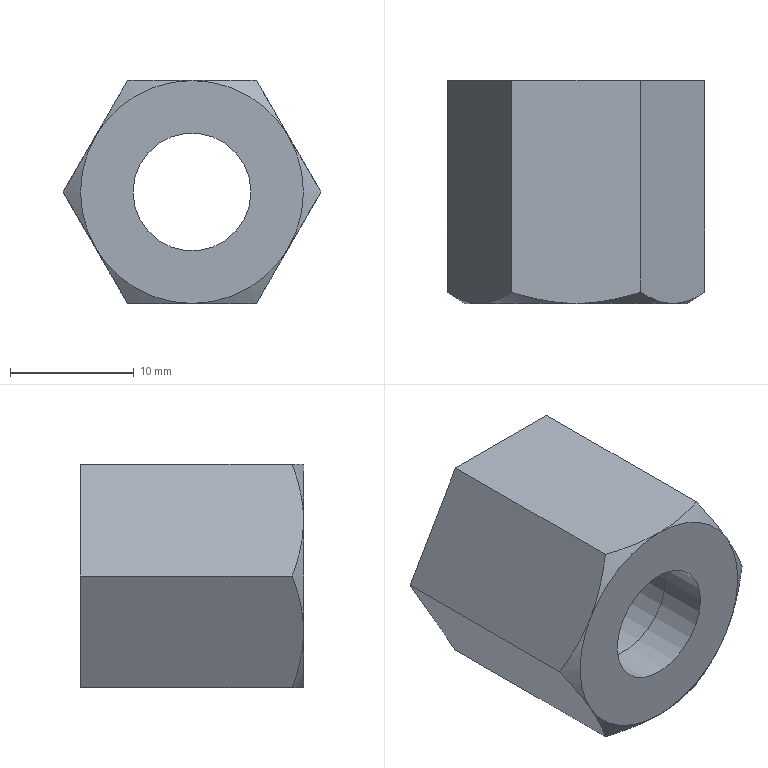Part | STEP file | 1-55.7 | 2 solids | 16 faces | box 20.785 x 18 x 18 mm | volume 3019 mm3 | plane 11 | cylinder 4 | cone 1 | commonest cylinder face diameters 9.5 x2 14 x2
STEP:
#1=CARTESIAN_POINT('',(0.,0.,0.));
#2=DIRECTION('',(0.,0.,1.));
#3=DIRECTION('',(1.,0.,0.));
#4=AXIS2_PLACEMENT_3D('',#1,#2,#3);
#5=CARTESIAN_POINT('',(7.,-14.,0.));
#6=VERTEX_POINT('',#5);
#7=CARTESIAN_POINT('',(0.,-14.,0.));
#8=DIRECTION('',(0.,-1.,0.));
#9=DIRECTION('',(1.,0.,0.));
#10=AXIS2_PLACEMENT_3D('',#7,#8,#9);
#11=CIRCLE('',#10,7.);
#12=CARTESIAN_POINT('',(-1.876,-14.,0.));
#13=DIRECTION('',(0.,-1.,0.));
#14=DIRECTION('',(1.,0.,0.));
#15=AXIS2_PLACEMENT_3D('',#12,#13,#14);
#16=PLANE('',#15);
#17=CARTESIAN_POINT('',(1.876,0.));
#18=DIRECTION('',(1.,0.));
#19=AXIS2_PLACEMENT_2D('',#17,#18);
#20=CIRCLE('',#19,7.);
#21=(GEOMETRIC_REPRESENTATION_CONTEXT(2)PARAMETRIC_REPRESENTATION_CONTEXT()REPRESENTATION_CONTEXT('',''));
#22=DEFINITIONAL_REPRESENTATION('',(#20),#21);
#23=PCURVE('',#16,#22);
#24=CARTESIAN_POINT('',(0.,-14.,0.));
#25=DIRECTION('',(0.,1.,0.));
#26=DIRECTION('',(1.,0.,0.));
#27=AXIS2_PLACEMENT_3D('',#24,#25,#26);
#28=CYLINDRICAL_SURFACE('',#27,7.);
#29=CARTESIAN_POINT('',(6.283,0.));
#30=DIRECTION('',(-1.,0.));
#31=VECTOR('',#30,1.);
#32=LINE('',#29,#31);
#33=(GEOMETRIC_REPRESENTATION_CONTEXT(2)PARAMETRIC_REPRESENTATION_CONTEXT()REPRESENTATION_CONTEXT('',''));
#34=DEFINITIONAL_REPRESENTATION('',(#32),#33);
#35=PCURVE('',#28,#34);
#36=SURFACE_CURVE('',#11,(#23,#35),.PCURVE_S1.);
#37=EDGE_CURVE('',#6,#6,#36,.T.);
#38=ORIENTED_EDGE('',*,*,#37,.T.);
#39=EDGE_LOOP('',(#38));
#40=FACE_BOUND('',#39,.T.);
#41=CARTESIAN_POINT('',(4.75,-14.,0.));
#42=VERTEX_POINT('',#41);
#43=CARTESIAN_POINT('',(0.,-14.,0.));
#44=DIRECTION('',(0.,1.,0.));
#45=DIRECTION('',(1.,0.,0.));
#46=AXIS2_PLACEMENT_3D('',#43,#44,#45);
#47=CIRCLE('',#46,4.75);
#48=CARTESIAN_POINT('',(6.626,0.));
#49=CARTESIAN_POINT('',(6.626,-8.227));
#50=CARTESIAN_POINT('',(-0.4994,-4.114));
#51=CARTESIAN_POINT('',(-7.624,0.));
#52=CARTESIAN_POINT('',(-0.4994,4.114));
#53=CARTESIAN_POINT('',(6.626,8.227));
#54=CARTESIAN_POINT('',(6.626,0.));
#55=(BOUNDED_CURVE()B_SPLINE_CURVE(2,(#48,#49,#50,#51,#52,#53,#54),.UNSPECIFIED.,.T.,.F.)B_SPLINE_CURVE_WITH_KNOTS((1,2,2,2,2,1),(-2.094,0.,2.094,4.189,6.283,8.378),.UNSPECIFIED.)CURVE()GEOMETRIC_REPRESENTATION_ITEM()RATIONAL_B_SPLINE_CURVE((1.,0.5,1.,0.5,1.,0.5,1.))REPRESENTATION_ITEM(''));
#56=(GEOMETRIC_REPRESENTATION_CONTEXT(2)PARAMETRIC_REPRESENTATION_CONTEXT()REPRESENTATION_CONTEXT('',''));
#57=DEFINITIONAL_REPRESENTATION('',(#55),#56);
#58=PCURVE('',#16,#57);
#59=CARTESIAN_POINT('',(0.,-14.,0.));
#60=DIRECTION('',(0.,1.,0.));
#61=DIRECTION('',(1.,0.,0.));
#62=AXIS2_PLACEMENT_3D('',#59,#60,#61);
#63=CYLINDRICAL_SURFACE('',#62,4.75);
#64=CARTESIAN_POINT('',(0.,0.));
#65=DIRECTION('',(1.,0.));
#66=VECTOR('',#65,1.);
#67=LINE('',#64,#66);
#68=(GEOMETRIC_REPRESENTATION_CONTEXT(2)PARAMETRIC_REPRESENTATION_CONTEXT()REPRESENTATION_CONTEXT('',''));
#69=DEFINITIONAL_REPRESENTATION('',(#67),#68);
#70=PCURVE('',#63,#69);
#71=SURFACE_CURVE('',#47,(#58,#70),.PCURVE_S1.);
#72=EDGE_CURVE('',#42,#42,#71,.T.);
#73=ORIENTED_EDGE('',*,*,#72,.T.);
#74=EDGE_LOOP('',(#73));
#75=FACE_BOUND('',#74,.T.);
#76=ADVANCED_FACE('',(#40,#75),#16,.T.);
#77=CARTESIAN_POINT('',(7.,-9.,0.));
#78=VERTEX_POINT('',#77);
#79=CARTESIAN_POINT('',(0.,-9.,0.));
#80=DIRECTION('',(0.,-1.,0.));
#81=DIRECTION('',(1.,0.,0.));
#82=AXIS2_PLACEMENT_3D('',#79,#80,#81);
#83=CIRCLE('',#82,7.);
#84=CARTESIAN_POINT('',(-1.876,-9.,0.));
#85=DIRECTION('',(0.,-1.,0.));
#86=DIRECTION('',(1.,0.,0.));
#87=AXIS2_PLACEMENT_3D('',#84,#85,#86);
#88=PLANE('',#87);
#89=CARTESIAN_POINT('',(1.876,0.));
#90=DIRECTION('',(1.,0.));
#91=AXIS2_PLACEMENT_2D('',#89,#90);
#92=CIRCLE('',#91,7.);
#93=(GEOMETRIC_REPRESENTATION_CONTEXT(2)PARAMETRIC_REPRESENTATION_CONTEXT()REPRESENTATION_CONTEXT('',''));
#94=DEFINITIONAL_REPRESENTATION('',(#92),#93);
#95=PCURVE('',#88,#94);
#96=CARTESIAN_POINT('',(6.283,5.));
#97=DIRECTION('',(-1.,0.));
#98=VECTOR('',#97,1.);
#99=LINE('',#96,#98);
#100=(GEOMETRIC_REPRESENTATION_CONTEXT(2)PARAMETRIC_REPRESENTATION_CONTEXT()REPRESENTATION_CONTEXT('',''));
#101=DEFINITIONAL_REPRESENTATION('',(#99),#100);
#102=PCURVE('',#28,#101);
#103=SURFACE_CURVE('',#83,(#95,#102),.PCURVE_S1.);
#104=EDGE_CURVE('',#78,#78,#103,.T.);
#105=ORIENTED_EDGE('',*,*,#104,.T.);
#106=EDGE_LOOP('',(#105));
#107=FACE_BOUND('',#106,.F.);
#108=CARTESIAN_POINT('',(4.75,-9.,0.));
#109=VERTEX_POINT('',#108);
#110=CARTESIAN_POINT('',(0.,-9.,0.));
#111=DIRECTION('',(0.,1.,0.));
#112=DIRECTION('',(1.,0.,0.));
#113=AXIS2_PLACEMENT_3D('',#110,#111,#112);
#114=CIRCLE('',#113,4.75);
#115=CARTESIAN_POINT('',(6.626,0.));
#116=CARTESIAN_POINT('',(6.626,-8.227));
#117=CARTESIAN_POINT('',(-0.4994,-4.114));
#118=CARTESIAN_POINT('',(-7.624,0.));
#119=CARTESIAN_POINT('',(-0.4994,4.114));
#120=CARTESIAN_POINT('',(6.626,8.227));
#121=CARTESIAN_POINT('',(6.626,0.));
#122=(BOUNDED_CURVE()B_SPLINE_CURVE(2,(#115,#116,#117,#118,#119,#120,#121),.UNSPECIFIED.,.T.,.F.)B_SPLINE_CURVE_WITH_KNOTS((1,2,2,2,2,1),(-2.094,0.,2.094,4.189,6.283,8.378),.UNSPECIFIED.)CURVE()GEOMETRIC_REPRESENTATION_ITEM()RATIONAL_B_SPLINE_CURVE((1.,0.5,1.,0.5,1.,0.5,1.))REPRESENTATION_ITEM(''));
#123=(GEOMETRIC_REPRESENTATION_CONTEXT(2)PARAMETRIC_REPRESENTATION_CONTEXT()REPRESENTATION_CONTEXT('',''));
#124=DEFINITIONAL_REPRESENTATION('',(#122),#123);
#125=PCURVE('',#88,#124);
#126=CARTESIAN_POINT('',(0.,5.));
#127=DIRECTION('',(1.,0.));
#128=VECTOR('',#127,1.);
#129=LINE('',#126,#128);
#130=(GEOMETRIC_REPRESENTATION_CONTEXT(2)PARAMETRIC_REPRESENTATION_CONTEXT()REPRESENTATION_CONTEXT('',''));
#131=DEFINITIONAL_REPRESENTATION('',(#129),#130);
#132=PCURVE('',#63,#131);
#133=SURFACE_CURVE('',#114,(#125,#132),.PCURVE_S1.);
#134=EDGE_CURVE('',#109,#109,#133,.T.);
#135=ORIENTED_EDGE('',*,*,#134,.T.);
#136=EDGE_LOOP('',(#135));
#137=FACE_BOUND('',#136,.F.);
#138=ADVANCED_FACE('',(#107,#137),#88,.F.);
#139=CARTESIAN_POINT('',(7.,-14.,0.));
#140=DIRECTION('',(0.,1.,0.));
#141=VECTOR('',#140,1.);
#142=LINE('',#139,#141);
#143=CARTESIAN_POINT('',(6.283,0.));
#144=DIRECTION('',(0.,1.));
#145=VECTOR('',#144,1.);
#146=LINE('',#143,#145);
#147=(GEOMETRIC_REPRESENTATION_CONTEXT(2)PARAMETRIC_REPRESENTATION_CONTEXT()REPRESENTATION_CONTEXT('',''));
#148=DEFINITIONAL_REPRESENTATION('',(#146),#147);
#149=PCURVE('',#28,#148);
#150=CARTESIAN_POINT('',(0.,0.));
#151=DIRECTION('',(0.,1.));
#152=VECTOR('',#151,1.);
#153=LINE('',#150,#152);
#154=(GEOMETRIC_REPRESENTATION_CONTEXT(2)PARAMETRIC_REPRESENTATION_CONTEXT()REPRESENTATION_CONTEXT('',''));
#155=DEFINITIONAL_REPRESENTATION('',(#153),#154);
#156=PCURVE('',#28,#155);
#157=SEAM_CURVE('',#142,(#149,#156),.PCURVE_S1.);
#158=EDGE_CURVE('',#6,#78,#157,.T.);
#159=ORIENTED_EDGE('',*,*,#158,.T.);
#160=ORIENTED_EDGE('',*,*,#104,.T.);
#161=ORIENTED_EDGE('',*,*,#158,.F.);
#162=ORIENTED_EDGE('',*,*,#37,.F.);
#163=EDGE_LOOP('',(#159,#160,#161,#162));
#164=FACE_BOUND('',#163,.T.);
#165=ADVANCED_FACE('',(#164),#28,.T.);
#166=ORIENTED_EDGE('',*,*,#72,.T.);
#167=CARTESIAN_POINT('',(4.75,-14.,0.));
#168=DIRECTION('',(0.,1.,0.));
#169=VECTOR('',#168,1.);
#170=LINE('',#167,#169);
#171=CARTESIAN_POINT('',(6.283,0.));
#172=DIRECTION('',(0.,1.));
#173=VECTOR('',#172,1.);
#174=LINE('',#171,#173);
#175=(GEOMETRIC_REPRESENTATION_CONTEXT(2)PARAMETRIC_REPRESENTATION_CONTEXT()REPRESENTATION_CONTEXT('',''));
#176=DEFINITIONAL_REPRESENTATION('',(#174),#175);
#177=PCURVE('',#63,#176);
#178=CARTESIAN_POINT('',(0.,0.));
#179=DIRECTION('',(0.,1.));
#180=VECTOR('',#179,1.);
#181=LINE('',#178,#180);
#182=(GEOMETRIC_REPRESENTATION_CONTEXT(2)PARAMETRIC_REPRESENTATION_CONTEXT()REPRESENTATION_CONTEXT('',''));
#183=DEFINITIONAL_REPRESENTATION('',(#181),#182);
#184=PCURVE('',#63,#183);
#185=SEAM_CURVE('',#170,(#177,#184),.PCURVE_S1.);
#186=EDGE_CURVE('',#42,#109,#185,.T.);
#187=ORIENTED_EDGE('',*,*,#186,.T.);
#188=ORIENTED_EDGE('',*,*,#134,.F.);
#189=ORIENTED_EDGE('',*,*,#186,.F.);
#190=EDGE_LOOP('',(#166,#187,#188,#189));
#191=FACE_BOUND('',#190,.F.);
#192=ADVANCED_FACE('',(#191),#63,.F.);
#193=CLOSED_SHELL('',(#76,#138,#165,#192));
#194=MANIFOLD_SOLID_BREP('',#193);
#195=CARTESIAN_POINT('',(-5.196,0.,9.));
#196=VERTEX_POINT('',#195);
#197=CARTESIAN_POINT('',(5.196,0.,9.));
#198=VERTEX_POINT('',#197);
#199=CARTESIAN_POINT('',(-5.196,0.,9.));
#200=DIRECTION('',(1.,0.,0.));
#201=VECTOR('',#200,1.);
#202=LINE('',#199,#201);
#203=CARTESIAN_POINT('',(0.,0.,-1.392));
#204=DIRECTION('',(0.,1.,0.));
#205=DIRECTION('',(1.,0.,0.));
#206=AXIS2_PLACEMENT_3D('',#203,#204,#205);
#207=PLANE('',#206);
#208=CARTESIAN_POINT('',(-5.196,-10.392));
#209=DIRECTION('',(1.,0.));
#210=VECTOR('',#209,1.);
#211=LINE('',#208,#210);
#212=(GEOMETRIC_REPRESENTATION_CONTEXT(2)PARAMETRIC_REPRESENTATION_CONTEXT()REPRESENTATION_CONTEXT('',''));
#213=DEFINITIONAL_REPRESENTATION('',(#211),#212);
#214=PCURVE('',#207,#213);
#215=CARTESIAN_POINT('',(0.,-9.,9.));
#216=DIRECTION('',(0.,0.,-1.));
#217=DIRECTION('',(1.,0.,0.));
#218=AXIS2_PLACEMENT_3D('',#215,#216,#217);
#219=PLANE('',#218);
#220=CARTESIAN_POINT('',(-5.196,-9.));
#221=DIRECTION('',(1.,0.));
#222=VECTOR('',#221,1.);
#223=LINE('',#220,#222);
#224=(GEOMETRIC_REPRESENTATION_CONTEXT(2)PARAMETRIC_REPRESENTATION_CONTEXT()REPRESENTATION_CONTEXT('',''));
#225=DEFINITIONAL_REPRESENTATION('',(#223),#224);
#226=PCURVE('',#219,#225);
#227=SURFACE_CURVE('',#202,(#214,#226),.PCURVE_S1.);
#228=EDGE_CURVE('',#196,#198,#227,.T.);
#229=ORIENTED_EDGE('',*,*,#228,.T.);
#230=CARTESIAN_POINT('',(10.392,0.,0.));
#231=VERTEX_POINT('',#230);
#232=CARTESIAN_POINT('',(5.196,0.,9.));
#233=DIRECTION('',(0.5,0.,-0.866));
#234=VECTOR('',#233,1.);
#235=LINE('',#232,#234);
#236=CARTESIAN_POINT('',(5.196,-10.392));
#237=DIRECTION('',(0.5,0.866));
#238=VECTOR('',#237,1.);
#239=LINE('',#236,#238);
#240=(GEOMETRIC_REPRESENTATION_CONTEXT(2)PARAMETRIC_REPRESENTATION_CONTEXT()REPRESENTATION_CONTEXT('',''));
#241=DEFINITIONAL_REPRESENTATION('',(#239),#240);
#242=PCURVE('',#207,#241);
#243=CARTESIAN_POINT('',(7.794,-9.,4.5));
#244=DIRECTION('',(-0.866,0.,-0.5));
#245=DIRECTION('',(0.5,0.,-0.866));
#246=AXIS2_PLACEMENT_3D('',#243,#244,#245);
#247=PLANE('',#246);
#248=CARTESIAN_POINT('',(-5.196,-9.));
#249=DIRECTION('',(1.,0.));
#250=VECTOR('',#249,1.);
#251=LINE('',#248,#250);
#252=(GEOMETRIC_REPRESENTATION_CONTEXT(2)PARAMETRIC_REPRESENTATION_CONTEXT()REPRESENTATION_CONTEXT('',''));
#253=DEFINITIONAL_REPRESENTATION('',(#251),#252);
#254=PCURVE('',#247,#253);
#255=SURFACE_CURVE('',#235,(#242,#254),.PCURVE_S1.);
#256=EDGE_CURVE('',#198,#231,#255,.T.);
#257=ORIENTED_EDGE('',*,*,#256,.T.);
#258=CARTESIAN_POINT('',(5.196,0.,-9.));
#259=VERTEX_POINT('',#258);
#260=CARTESIAN_POINT('',(10.392,0.,0.));
#261=DIRECTION('',(-0.5,0.,-0.866));
#262=VECTOR('',#261,1.);
#263=LINE('',#260,#262);
#264=CARTESIAN_POINT('',(10.392,-1.392));
#265=DIRECTION('',(-0.5,0.866));
#266=VECTOR('',#265,1.);
#267=LINE('',#264,#266);
#268=(GEOMETRIC_REPRESENTATION_CONTEXT(2)PARAMETRIC_REPRESENTATION_CONTEXT()REPRESENTATION_CONTEXT('',''));
#269=DEFINITIONAL_REPRESENTATION('',(#267),#268);
#270=PCURVE('',#207,#269);
#271=CARTESIAN_POINT('',(7.794,-9.,-4.5));
#272=DIRECTION('',(-0.866,0.,0.5));
#273=DIRECTION('',(-0.5,0.,-0.866));
#274=AXIS2_PLACEMENT_3D('',#271,#272,#273);
#275=PLANE('',#274);
#276=CARTESIAN_POINT('',(-5.196,-9.));
#277=DIRECTION('',(1.,0.));
#278=VECTOR('',#277,1.);
#279=LINE('',#276,#278);
#280=(GEOMETRIC_REPRESENTATION_CONTEXT(2)PARAMETRIC_REPRESENTATION_CONTEXT()REPRESENTATION_CONTEXT('',''));
#281=DEFINITIONAL_REPRESENTATION('',(#279),#280);
#282=PCURVE('',#275,#281);
#283=SURFACE_CURVE('',#263,(#270,#282),.PCURVE_S1.);
#284=EDGE_CURVE('',#231,#259,#283,.T.);
#285=ORIENTED_EDGE('',*,*,#284,.T.);
#286=CARTESIAN_POINT('',(-5.196,0.,-9.));
#287=VERTEX_POINT('',#286);
#288=CARTESIAN_POINT('',(5.196,0.,-9.));
#289=DIRECTION('',(-1.,0.,0.));
#290=VECTOR('',#289,1.);
#291=LINE('',#288,#290);
#292=CARTESIAN_POINT('',(5.196,7.608));
#293=DIRECTION('',(-1.,0.));
#294=VECTOR('',#293,1.);
#295=LINE('',#292,#294);
#296=(GEOMETRIC_REPRESENTATION_CONTEXT(2)PARAMETRIC_REPRESENTATION_CONTEXT()REPRESENTATION_CONTEXT('',''));
#297=DEFINITIONAL_REPRESENTATION('',(#295),#296);
#298=PCURVE('',#207,#297);
#299=CARTESIAN_POINT('',(0.,-9.,-9.));
#300=DIRECTION('',(0.,0.,1.));
#301=DIRECTION('',(-1.,0.,0.));
#302=AXIS2_PLACEMENT_3D('',#299,#300,#301);
#303=PLANE('',#302);
#304=CARTESIAN_POINT('',(-5.196,-9.));
#305=DIRECTION('',(1.,0.));
#306=VECTOR('',#305,1.);
#307=LINE('',#304,#306);
#308=(GEOMETRIC_REPRESENTATION_CONTEXT(2)PARAMETRIC_REPRESENTATION_CONTEXT()REPRESENTATION_CONTEXT('',''));
#309=DEFINITIONAL_REPRESENTATION('',(#307),#308);
#310=PCURVE('',#303,#309);
#311=SURFACE_CURVE('',#291,(#298,#310),.PCURVE_S1.);
#312=EDGE_CURVE('',#259,#287,#311,.T.);
#313=ORIENTED_EDGE('',*,*,#312,.T.);
#314=CARTESIAN_POINT('',(-10.392,0.,0.));
#315=VERTEX_POINT('',#314);
#316=CARTESIAN_POINT('',(-5.196,0.,-9.));
#317=DIRECTION('',(-0.5,0.,0.866));
#318=VECTOR('',#317,1.);
#319=LINE('',#316,#318);
#320=CARTESIAN_POINT('',(-5.196,7.608));
#321=DIRECTION('',(-0.5,-0.866));
#322=VECTOR('',#321,1.);
#323=LINE('',#320,#322);
#324=(GEOMETRIC_REPRESENTATION_CONTEXT(2)PARAMETRIC_REPRESENTATION_CONTEXT()REPRESENTATION_CONTEXT('',''));
#325=DEFINITIONAL_REPRESENTATION('',(#323),#324);
#326=PCURVE('',#207,#325);
#327=CARTESIAN_POINT('',(-7.794,-9.,-4.5));
#328=DIRECTION('',(0.866,0.,0.5));
#329=DIRECTION('',(-0.5,0.,0.866));
#330=AXIS2_PLACEMENT_3D('',#327,#328,#329);
#331=PLANE('',#330);
#332=CARTESIAN_POINT('',(-5.196,-9.));
#333=DIRECTION('',(1.,0.));
#334=VECTOR('',#333,1.);
#335=LINE('',#332,#334);
#336=(GEOMETRIC_REPRESENTATION_CONTEXT(2)PARAMETRIC_REPRESENTATION_CONTEXT()REPRESENTATION_CONTEXT('',''));
#337=DEFINITIONAL_REPRESENTATION('',(#335),#336);
#338=PCURVE('',#331,#337);
#339=SURFACE_CURVE('',#319,(#326,#338),.PCURVE_S1.);
#340=EDGE_CURVE('',#287,#315,#339,.T.);
#341=ORIENTED_EDGE('',*,*,#340,.T.);
#342=CARTESIAN_POINT('',(-10.392,0.,0.));
#343=DIRECTION('',(0.5,0.,0.866));
#344=VECTOR('',#343,1.);
#345=LINE('',#342,#344);
#346=CARTESIAN_POINT('',(-10.392,-1.392));
#347=DIRECTION('',(0.5,-0.866));
#348=VECTOR('',#347,1.);
#349=LINE('',#346,#348);
#350=(GEOMETRIC_REPRESENTATION_CONTEXT(2)PARAMETRIC_REPRESENTATION_CONTEXT()REPRESENTATION_CONTEXT('',''));
#351=DEFINITIONAL_REPRESENTATION('',(#349),#350);
#352=PCURVE('',#207,#351);
#353=CARTESIAN_POINT('',(-7.794,-9.,4.5));
#354=DIRECTION('',(0.866,0.,-0.5));
#355=DIRECTION('',(0.5,0.,0.866));
#356=AXIS2_PLACEMENT_3D('',#353,#354,#355);
#357=PLANE('',#356);
#358=CARTESIAN_POINT('',(-5.196,-9.));
#359=DIRECTION('',(1.,0.));
#360=VECTOR('',#359,1.);
#361=LINE('',#358,#360);
#362=(GEOMETRIC_REPRESENTATION_CONTEXT(2)PARAMETRIC_REPRESENTATION_CONTEXT()REPRESENTATION_CONTEXT('',''));
#363=DEFINITIONAL_REPRESENTATION('',(#361),#362);
#364=PCURVE('',#357,#363);
#365=SURFACE_CURVE('',#345,(#352,#364),.PCURVE_S1.);
#366=EDGE_CURVE('',#315,#196,#365,.T.);
#367=ORIENTED_EDGE('',*,*,#366,.T.);
#368=EDGE_LOOP('',(#229,#257,#285,#313,#341,#367));
#369=FACE_BOUND('',#368,.T.);
#370=CARTESIAN_POINT('',(7.,0.,0.));
#371=VERTEX_POINT('',#370);
#372=CARTESIAN_POINT('',(0.,0.,0.));
#373=DIRECTION('',(0.,-1.,0.));
#374=DIRECTION('',(1.,0.,0.));
#375=AXIS2_PLACEMENT_3D('',#372,#373,#374);
#376=CIRCLE('',#375,7.);
#377=CARTESIAN_POINT('',(7.,-1.392));
#378=CARTESIAN_POINT('',(7.,-13.517));
#379=CARTESIAN_POINT('',(-3.5,-7.454));
#380=CARTESIAN_POINT('',(-14.,-1.392));
#381=CARTESIAN_POINT('',(-3.5,4.67));
#382=CARTESIAN_POINT('',(7.,10.732));
#383=CARTESIAN_POINT('',(7.,-1.392));
#384=(BOUNDED_CURVE()B_SPLINE_CURVE(2,(#377,#378,#379,#380,#381,#382,#383),.UNSPECIFIED.,.T.,.F.)B_SPLINE_CURVE_WITH_KNOTS((1,2,2,2,2,1),(-2.094,0.,2.094,4.189,6.283,8.378),.UNSPECIFIED.)CURVE()GEOMETRIC_REPRESENTATION_ITEM()RATIONAL_B_SPLINE_CURVE((1.,0.5,1.,0.5,1.,0.5,1.))REPRESENTATION_ITEM(''));
#385=(GEOMETRIC_REPRESENTATION_CONTEXT(2)PARAMETRIC_REPRESENTATION_CONTEXT()REPRESENTATION_CONTEXT('',''));
#386=DEFINITIONAL_REPRESENTATION('',(#384),#385);
#387=PCURVE('',#207,#386);
#388=CARTESIAN_POINT('',(0.,0.,0.));
#389=DIRECTION('',(0.,-1.,0.));
#390=DIRECTION('',(1.,0.,0.));
#391=AXIS2_PLACEMENT_3D('',#388,#389,#390);
#392=CYLINDRICAL_SURFACE('',#391,7.);
#393=CARTESIAN_POINT('',(0.,0.));
#394=DIRECTION('',(1.,0.));
#395=VECTOR('',#394,1.);
#396=LINE('',#393,#395);
#397=(GEOMETRIC_REPRESENTATION_CONTEXT(2)PARAMETRIC_REPRESENTATION_CONTEXT()REPRESENTATION_CONTEXT('',''));
#398=DEFINITIONAL_REPRESENTATION('',(#396),#397);
#399=PCURVE('',#392,#398);
#400=SURFACE_CURVE('',#376,(#387,#399),.PCURVE_S1.);
#401=EDGE_CURVE('',#371,#371,#400,.T.);
#402=ORIENTED_EDGE('',*,*,#401,.T.);
#403=EDGE_LOOP('',(#402));
#404=FACE_BOUND('',#403,.T.);
#405=ADVANCED_FACE('',(#369,#404),#207,.T.);
#406=ORIENTED_EDGE('',*,*,#401,.T.);
#407=CARTESIAN_POINT('',(7.,-14.,0.));
#408=VERTEX_POINT('',#407);
#409=CARTESIAN_POINT('',(7.,0.,0.));
#410=DIRECTION('',(0.,-1.,0.));
#411=VECTOR('',#410,1.);
#412=LINE('',#409,#411);
#413=CARTESIAN_POINT('',(6.283,0.));
#414=DIRECTION('',(0.,1.));
#415=VECTOR('',#414,1.);
#416=LINE('',#413,#415);
#417=(GEOMETRIC_REPRESENTATION_CONTEXT(2)PARAMETRIC_REPRESENTATION_CONTEXT()REPRESENTATION_CONTEXT('',''));
#418=DEFINITIONAL_REPRESENTATION('',(#416),#417);
#419=PCURVE('',#392,#418);
#420=CARTESIAN_POINT('',(0.,0.));
#421=DIRECTION('',(0.,1.));
#422=VECTOR('',#421,1.);
#423=LINE('',#420,#422);
#424=(GEOMETRIC_REPRESENTATION_CONTEXT(2)PARAMETRIC_REPRESENTATION_CONTEXT()REPRESENTATION_CONTEXT('',''));
#425=DEFINITIONAL_REPRESENTATION('',(#423),#424);
#426=PCURVE('',#392,#425);
#427=SEAM_CURVE('',#412,(#419,#426),.PCURVE_S1.);
#428=EDGE_CURVE('',#371,#408,#427,.T.);
#429=ORIENTED_EDGE('',*,*,#428,.T.);
#430=CARTESIAN_POINT('',(0.,-14.,0.));
#431=DIRECTION('',(0.,-1.,0.));
#432=DIRECTION('',(1.,0.,0.));
#433=AXIS2_PLACEMENT_3D('',#430,#431,#432);
#434=CIRCLE('',#433,7.);
#435=CARTESIAN_POINT('',(0.,14.));
#436=DIRECTION('',(1.,0.));
#437=VECTOR('',#436,1.);
#438=LINE('',#435,#437);
#439=(GEOMETRIC_REPRESENTATION_CONTEXT(2)PARAMETRIC_REPRESENTATION_CONTEXT()REPRESENTATION_CONTEXT('',''));
#440=DEFINITIONAL_REPRESENTATION('',(#438),#439);
#441=PCURVE('',#392,#440);
#442=CARTESIAN_POINT('',(-1.876,-14.,0.));
#443=DIRECTION('',(0.,-1.,0.));
#444=DIRECTION('',(1.,0.,0.));
#445=AXIS2_PLACEMENT_3D('',#442,#443,#444);
#446=PLANE('',#445);
#447=CARTESIAN_POINT('',(1.876,0.));
#448=DIRECTION('',(1.,0.));
#449=AXIS2_PLACEMENT_2D('',#447,#448);
#450=CIRCLE('',#449,7.);
#451=(GEOMETRIC_REPRESENTATION_CONTEXT(2)PARAMETRIC_REPRESENTATION_CONTEXT()REPRESENTATION_CONTEXT('',''));
#452=DEFINITIONAL_REPRESENTATION('',(#450),#451);
#453=PCURVE('',#446,#452);
#454=SURFACE_CURVE('',#434,(#441,#453),.PCURVE_S1.);
#455=EDGE_CURVE('',#408,#408,#454,.T.);
#456=ORIENTED_EDGE('',*,*,#455,.F.);
#457=ORIENTED_EDGE('',*,*,#428,.F.);
#458=EDGE_LOOP('',(#406,#429,#456,#457));
#459=FACE_BOUND('',#458,.F.);
#460=ADVANCED_FACE('',(#459),#392,.F.);
#461=ORIENTED_EDGE('',*,*,#455,.T.);
#462=EDGE_LOOP('',(#461));
#463=FACE_BOUND('',#462,.F.);
#464=CARTESIAN_POINT('',(4.75,-14.,0.));
#465=VERTEX_POINT('',#464);
#466=CARTESIAN_POINT('',(0.,-14.,0.));
#467=DIRECTION('',(0.,1.,0.));
#468=DIRECTION('',(1.,0.,0.));
#469=AXIS2_PLACEMENT_3D('',#466,#467,#468);
#470=CIRCLE('',#469,4.75);
#471=CARTESIAN_POINT('',(6.626,0.));
#472=CARTESIAN_POINT('',(6.626,-8.227));
#473=CARTESIAN_POINT('',(-0.4994,-4.114));
#474=CARTESIAN_POINT('',(-7.624,0.));
#475=CARTESIAN_POINT('',(-0.4994,4.114));
#476=CARTESIAN_POINT('',(6.626,8.227));
#477=CARTESIAN_POINT('',(6.626,0.));
#478=(BOUNDED_CURVE()B_SPLINE_CURVE(2,(#471,#472,#473,#474,#475,#476,#477),.UNSPECIFIED.,.T.,.F.)B_SPLINE_CURVE_WITH_KNOTS((1,2,2,2,2,1),(-2.094,0.,2.094,4.189,6.283,8.378),.UNSPECIFIED.)CURVE()GEOMETRIC_REPRESENTATION_ITEM()RATIONAL_B_SPLINE_CURVE((1.,0.5,1.,0.5,1.,0.5,1.))REPRESENTATION_ITEM(''));
#479=(GEOMETRIC_REPRESENTATION_CONTEXT(2)PARAMETRIC_REPRESENTATION_CONTEXT()REPRESENTATION_CONTEXT('',''));
#480=DEFINITIONAL_REPRESENTATION('',(#478),#479);
#481=PCURVE('',#446,#480);
#482=CARTESIAN_POINT('',(0.,0.,0.));
#483=DIRECTION('',(0.,-1.,0.));
#484=DIRECTION('',(1.,0.,0.));
#485=AXIS2_PLACEMENT_3D('',#482,#483,#484);
#486=CYLINDRICAL_SURFACE('',#485,4.75);
#487=CARTESIAN_POINT('',(6.283,14.));
#488=DIRECTION('',(-1.,0.));
#489=VECTOR('',#488,1.);
#490=LINE('',#487,#489);
#491=(GEOMETRIC_REPRESENTATION_CONTEXT(2)PARAMETRIC_REPRESENTATION_CONTEXT()REPRESENTATION_CONTEXT('',''));
#492=DEFINITIONAL_REPRESENTATION('',(#490),#491);
#493=PCURVE('',#486,#492);
#494=SURFACE_CURVE('',#470,(#481,#493),.PCURVE_S1.);
#495=EDGE_CURVE('',#465,#465,#494,.T.);
#496=ORIENTED_EDGE('',*,*,#495,.T.);
#497=EDGE_LOOP('',(#496));
#498=FACE_BOUND('',#497,.F.);
#499=ADVANCED_FACE('',(#463,#498),#446,.F.);
#500=CARTESIAN_POINT('',(4.75,-18.,0.));
#501=VERTEX_POINT('',#500);
#502=CARTESIAN_POINT('',(0.,-18.,0.));
#503=DIRECTION('',(0.,-1.,0.));
#504=DIRECTION('',(1.,0.,0.));
#505=AXIS2_PLACEMENT_3D('',#502,#503,#504);
#506=CIRCLE('',#505,4.75);
#507=CARTESIAN_POINT('',(0.,18.));
#508=DIRECTION('',(1.,0.));
#509=VECTOR('',#508,1.);
#510=LINE('',#507,#509);
#511=(GEOMETRIC_REPRESENTATION_CONTEXT(2)PARAMETRIC_REPRESENTATION_CONTEXT()REPRESENTATION_CONTEXT('',''));
#512=DEFINITIONAL_REPRESENTATION('',(#510),#511);
#513=PCURVE('',#486,#512);
#514=CARTESIAN_POINT('',(0.,-18.,-1.392));
#515=DIRECTION('',(0.,1.,0.));
#516=DIRECTION('',(1.,0.,0.));
#517=AXIS2_PLACEMENT_3D('',#514,#515,#516);
#518=PLANE('',#517);
#519=CARTESIAN_POINT('',(4.75,-1.392));
#520=CARTESIAN_POINT('',(4.75,-9.62));
#521=CARTESIAN_POINT('',(-2.375,-5.506));
#522=CARTESIAN_POINT('',(-9.5,-1.392));
#523=CARTESIAN_POINT('',(-2.375,2.721));
#524=CARTESIAN_POINT('',(4.75,6.835));
#525=CARTESIAN_POINT('',(4.75,-1.392));
#526=(BOUNDED_CURVE()B_SPLINE_CURVE(2,(#519,#520,#521,#522,#523,#524,#525),.UNSPECIFIED.,.T.,.F.)B_SPLINE_CURVE_WITH_KNOTS((1,2,2,2,2,1),(-2.094,0.,2.094,4.189,6.283,8.378),.UNSPECIFIED.)CURVE()GEOMETRIC_REPRESENTATION_ITEM()RATIONAL_B_SPLINE_CURVE((1.,0.5,1.,0.5,1.,0.5,1.))REPRESENTATION_ITEM(''));
#527=(GEOMETRIC_REPRESENTATION_CONTEXT(2)PARAMETRIC_REPRESENTATION_CONTEXT()REPRESENTATION_CONTEXT('',''));
#528=DEFINITIONAL_REPRESENTATION('',(#526),#527);
#529=PCURVE('',#518,#528);
#530=SURFACE_CURVE('',#506,(#513,#529),.PCURVE_S1.);
#531=EDGE_CURVE('',#501,#501,#530,.T.);
#532=ORIENTED_EDGE('',*,*,#531,.F.);
#533=CARTESIAN_POINT('',(4.75,-14.,0.));
#534=DIRECTION('',(0.,-1.,0.));
#535=VECTOR('',#534,1.);
#536=LINE('',#533,#535);
#537=CARTESIAN_POINT('',(0.,14.));
#538=DIRECTION('',(0.,1.));
#539=VECTOR('',#538,1.);
#540=LINE('',#537,#539);
#541=(GEOMETRIC_REPRESENTATION_CONTEXT(2)PARAMETRIC_REPRESENTATION_CONTEXT()REPRESENTATION_CONTEXT('',''));
#542=DEFINITIONAL_REPRESENTATION('',(#540),#541);
#543=PCURVE('',#486,#542);
#544=CARTESIAN_POINT('',(6.283,14.));
#545=DIRECTION('',(0.,1.));
#546=VECTOR('',#545,1.);
#547=LINE('',#544,#546);
#548=(GEOMETRIC_REPRESENTATION_CONTEXT(2)PARAMETRIC_REPRESENTATION_CONTEXT()REPRESENTATION_CONTEXT('',''));
#549=DEFINITIONAL_REPRESENTATION('',(#547),#548);
#550=PCURVE('',#486,#549);
#551=SEAM_CURVE('',#536,(#543,#550),.PCURVE_S1.);
#552=EDGE_CURVE('',#465,#501,#551,.T.);
#553=ORIENTED_EDGE('',*,*,#552,.F.);
#554=ORIENTED_EDGE('',*,*,#495,.F.);
#555=ORIENTED_EDGE('',*,*,#552,.T.);
#556=EDGE_LOOP('',(#532,#553,#554,#555));
#557=FACE_BOUND('',#556,.F.);
#558=ADVANCED_FACE('',(#557),#486,.F.);
#559=ORIENTED_EDGE('',*,*,#228,.T.);
#560=CARTESIAN_POINT('',(5.196,-17.085,9.));
#561=VERTEX_POINT('',#560);
#562=CARTESIAN_POINT('',(5.196,0.,9.));
#563=DIRECTION('',(0.,-1.,0.));
#564=VECTOR('',#563,1.);
#565=LINE('',#562,#564);
#566=CARTESIAN_POINT('',(5.196,-9.));
#567=DIRECTION('',(0.,1.));
#568=VECTOR('',#567,1.);
#569=LINE('',#566,#568);
#570=(GEOMETRIC_REPRESENTATION_CONTEXT(2)PARAMETRIC_REPRESENTATION_CONTEXT()REPRESENTATION_CONTEXT('',''));
#571=DEFINITIONAL_REPRESENTATION('',(#569),#570);
#572=PCURVE('',#219,#571);
#573=CARTESIAN_POINT('',(-5.196,-9.));
#574=DIRECTION('',(0.,1.));
#575=VECTOR('',#574,1.);
#576=LINE('',#573,#575);
#577=(GEOMETRIC_REPRESENTATION_CONTEXT(2)PARAMETRIC_REPRESENTATION_CONTEXT()REPRESENTATION_CONTEXT('',''));
#578=DEFINITIONAL_REPRESENTATION('',(#576),#577);
#579=PCURVE('',#247,#578);
#580=SURFACE_CURVE('',#565,(#572,#579),.PCURVE_S1.);
#581=EDGE_CURVE('',#198,#561,#580,.T.);
#582=ORIENTED_EDGE('',*,*,#581,.T.);
#583=CARTESIAN_POINT('',(0.,-17.996,9.));
#584=VERTEX_POINT('',#583);
#585=CARTESIAN_POINT('',(5.196,-17.085,9.));
#586=CARTESIAN_POINT('',(2.412,-17.991,9.));
#587=CARTESIAN_POINT('',(0.,-17.991,9.));
#588=(BOUNDED_CURVE()B_SPLINE_CURVE(2,(#585,#586,#587),.UNSPECIFIED.,.F.,.F.)B_SPLINE_CURVE_WITH_KNOTS((3,3),(0.,1.),.PIECEWISE_BEZIER_KNOTS.)CURVE()GEOMETRIC_REPRESENTATION_ITEM()RATIONAL_B_SPLINE_CURVE((1.426,1.537,1.537))REPRESENTATION_ITEM(''));
#589=CARTESIAN_POINT('',(5.196,8.085));
#590=CARTESIAN_POINT('',(2.412,8.991));
#591=CARTESIAN_POINT('',(0.,8.991));
#592=(BOUNDED_CURVE()B_SPLINE_CURVE(2,(#589,#590,#591),.UNSPECIFIED.,.F.,.F.)B_SPLINE_CURVE_WITH_KNOTS((3,3),(0.,1.),.PIECEWISE_BEZIER_KNOTS.)CURVE()GEOMETRIC_REPRESENTATION_ITEM()RATIONAL_B_SPLINE_CURVE((1.426,1.537,1.537))REPRESENTATION_ITEM(''));
#593=(GEOMETRIC_REPRESENTATION_CONTEXT(2)PARAMETRIC_REPRESENTATION_CONTEXT()REPRESENTATION_CONTEXT('',''));
#594=DEFINITIONAL_REPRESENTATION('',(#592),#593);
#595=PCURVE('',#219,#594);
#596=CARTESIAN_POINT('',(0.,-18.,0.));
#597=DIRECTION('',(0.,1.,0.));
#598=DIRECTION('',(0.,0.,1.));
#599=AXIS2_PLACEMENT_3D('',#596,#597,#598);
#600=CONICAL_SURFACE('',#599,8.986,0.994);
#601=CARTESIAN_POINT('',(0.5236,0.9146));
#602=CARTESIAN_POINT('',(0.516,0.8851));
#603=CARTESIAN_POINT('',(0.5008,0.8277));
#604=CARTESIAN_POINT('',(0.4779,0.7467));
#605=CARTESIAN_POINT('',(0.4548,0.6706));
#606=CARTESIAN_POINT('',(0.4317,0.5993));
#607=CARTESIAN_POINT('',(0.4084,0.5326));
#608=CARTESIAN_POINT('',(0.3849,0.4704));
#609=CARTESIAN_POINT('',(0.3614,0.4125));
#610=CARTESIAN_POINT('',(0.3378,0.3588));
#611=CARTESIAN_POINT('',(0.3141,0.3093));
#612=CARTESIAN_POINT('',(0.2903,0.2638));
#613=CARTESIAN_POINT('',(0.2664,0.2222));
#614=CARTESIAN_POINT('',(0.2424,0.1846));
#615=CARTESIAN_POINT('',(0.2184,0.1507));
#616=CARTESIAN_POINT('',(0.1943,0.1205));
#617=CARTESIAN_POINT('',(0.1701,0.094));
#618=CARTESIAN_POINT('',(0.1459,0.07114));
#619=CARTESIAN_POINT('',(0.1217,0.05186));
#620=CARTESIAN_POINT('',(0.09736,0.03614));
#621=CARTESIAN_POINT('',(0.07305,0.02394));
#622=CARTESIAN_POINT('',(0.04871,0.01524));
#623=CARTESIAN_POINT('',(0.02436,0.01002));
#624=CARTESIAN_POINT('',(0.00812,0.008865));
#625=CARTESIAN_POINT('',(0.,0.008865));
#626=B_SPLINE_CURVE_WITH_KNOTS('',3,(#601,#602,#603,#604,#605,#606,#607,#608,#609,#610,#611,#612,#613,#614,#615,#616,#617,#618,#619,#620,#621,#622,#623,#624,#625),.UNSPECIFIED.,.F.,.F.,(4,1,1,1,1,1,1,1,1,1,1,1,1,1,1,1,1,1,1,1,1,1,4),(0.,0.04545,0.09091,0.1364,0.1818,0.2273,0.2727,0.3182,0.3636,0.4091,0.4545,0.5,0.5455,0.5909,0.6364,0.6818,0.7273,0.7727,0.8182,0.8636,0.9091,0.9545,1.),.QUASI_UNIFORM_KNOTS.);
#627=(GEOMETRIC_REPRESENTATION_CONTEXT(2)PARAMETRIC_REPRESENTATION_CONTEXT()REPRESENTATION_CONTEXT('',''));
#628=DEFINITIONAL_REPRESENTATION('',(#626),#627);
#629=PCURVE('',#600,#628);
#630=SURFACE_CURVE('',#588,(#595,#629),.PCURVE_S1.);
#631=EDGE_CURVE('',#561,#584,#630,.T.);
#632=ORIENTED_EDGE('',*,*,#631,.T.);
#633=CARTESIAN_POINT('',(-5.196,-17.085,9.));
#634=VERTEX_POINT('',#633);
#635=CARTESIAN_POINT('',(0.,-17.991,9.));
#636=CARTESIAN_POINT('',(-2.412,-17.991,9.));
#637=CARTESIAN_POINT('',(-5.196,-17.085,9.));
#638=(BOUNDED_CURVE()B_SPLINE_CURVE(2,(#635,#636,#637),.UNSPECIFIED.,.F.,.F.)B_SPLINE_CURVE_WITH_KNOTS((3,3),(0.,1.),.PIECEWISE_BEZIER_KNOTS.)CURVE()GEOMETRIC_REPRESENTATION_ITEM()RATIONAL_B_SPLINE_CURVE((1.537,1.537,1.426))REPRESENTATION_ITEM(''));
#639=CARTESIAN_POINT('',(0.,8.991));
#640=CARTESIAN_POINT('',(-2.412,8.991));
#641=CARTESIAN_POINT('',(-5.196,8.085));
#642=(BOUNDED_CURVE()B_SPLINE_CURVE(2,(#639,#640,#641),.UNSPECIFIED.,.F.,.F.)B_SPLINE_CURVE_WITH_KNOTS((3,3),(0.,1.),.PIECEWISE_BEZIER_KNOTS.)CURVE()GEOMETRIC_REPRESENTATION_ITEM()RATIONAL_B_SPLINE_CURVE((1.537,1.537,1.426))REPRESENTATION_ITEM(''));
#643=(GEOMETRIC_REPRESENTATION_CONTEXT(2)PARAMETRIC_REPRESENTATION_CONTEXT()REPRESENTATION_CONTEXT('',''));
#644=DEFINITIONAL_REPRESENTATION('',(#642),#643);
#645=PCURVE('',#219,#644);
#646=CARTESIAN_POINT('',(6.283,0.008865));
#647=CARTESIAN_POINT('',(6.275,0.008865));
#648=CARTESIAN_POINT('',(6.259,0.01002));
#649=CARTESIAN_POINT('',(6.234,0.01524));
#650=CARTESIAN_POINT('',(6.21,0.02394));
#651=CARTESIAN_POINT('',(6.186,0.03614));
#652=CARTESIAN_POINT('',(6.162,0.05186));
#653=CARTESIAN_POINT('',(6.137,0.07114));
#654=CARTESIAN_POINT('',(6.113,0.094));
#655=CARTESIAN_POINT('',(6.089,0.1205));
#656=CARTESIAN_POINT('',(6.065,0.1507));
#657=CARTESIAN_POINT('',(6.041,0.1846));
#658=CARTESIAN_POINT('',(6.017,0.2222));
#659=CARTESIAN_POINT('',(5.993,0.2638));
#660=CARTESIAN_POINT('',(5.969,0.3093));
#661=CARTESIAN_POINT('',(5.945,0.3588));
#662=CARTESIAN_POINT('',(5.922,0.4125));
#663=CARTESIAN_POINT('',(5.898,0.4704));
#664=CARTESIAN_POINT('',(5.875,0.5326));
#665=CARTESIAN_POINT('',(5.852,0.5993));
#666=CARTESIAN_POINT('',(5.828,0.6706));
#667=CARTESIAN_POINT('',(5.805,0.7467));
#668=CARTESIAN_POINT('',(5.782,0.8277));
#669=CARTESIAN_POINT('',(5.767,0.8851));
#670=CARTESIAN_POINT('',(5.76,0.9146));
#671=B_SPLINE_CURVE_WITH_KNOTS('',3,(#646,#647,#648,#649,#650,#651,#652,#653,#654,#655,#656,#657,#658,#659,#660,#661,#662,#663,#664,#665,#666,#667,#668,#669,#670),.UNSPECIFIED.,.F.,.F.,(4,1,1,1,1,1,1,1,1,1,1,1,1,1,1,1,1,1,1,1,1,1,4),(0.,0.04545,0.09091,0.1364,0.1818,0.2273,0.2727,0.3182,0.3636,0.4091,0.4545,0.5,0.5455,0.5909,0.6364,0.6818,0.7273,0.7727,0.8182,0.8636,0.9091,0.9545,1.),.QUASI_UNIFORM_KNOTS.);
#672=(GEOMETRIC_REPRESENTATION_CONTEXT(2)PARAMETRIC_REPRESENTATION_CONTEXT()REPRESENTATION_CONTEXT('',''));
#673=DEFINITIONAL_REPRESENTATION('',(#671),#672);
#674=PCURVE('',#600,#673);
#675=SURFACE_CURVE('',#638,(#645,#674),.PCURVE_S1.);
#676=EDGE_CURVE('',#584,#634,#675,.T.);
#677=ORIENTED_EDGE('',*,*,#676,.T.);
#678=CARTESIAN_POINT('',(-5.196,0.,9.));
#679=DIRECTION('',(0.,-1.,0.));
#680=VECTOR('',#679,1.);
#681=LINE('',#678,#680);
#682=CARTESIAN_POINT('',(-5.196,-9.));
#683=DIRECTION('',(0.,1.));
#684=VECTOR('',#683,1.);
#685=LINE('',#682,#684);
#686=(GEOMETRIC_REPRESENTATION_CONTEXT(2)PARAMETRIC_REPRESENTATION_CONTEXT()REPRESENTATION_CONTEXT('',''));
#687=DEFINITIONAL_REPRESENTATION('',(#685),#686);
#688=PCURVE('',#219,#687);
#689=CARTESIAN_POINT('',(5.196,-9.));
#690=DIRECTION('',(0.,1.));
#691=VECTOR('',#690,1.);
#692=LINE('',#689,#691);
#693=(GEOMETRIC_REPRESENTATION_CONTEXT(2)PARAMETRIC_REPRESENTATION_CONTEXT()REPRESENTATION_CONTEXT('',''));
#694=DEFINITIONAL_REPRESENTATION('',(#692),#693);
#695=PCURVE('',#357,#694);
#696=SURFACE_CURVE('',#681,(#688,#695),.PCURVE_S1.);
#697=EDGE_CURVE('',#196,#634,#696,.T.);
#698=ORIENTED_EDGE('',*,*,#697,.F.);
#699=EDGE_LOOP('',(#559,#582,#632,#677,#698));
#700=FACE_BOUND('',#699,.F.);
#701=ADVANCED_FACE('',(#700),#219,.F.);
#702=ORIENTED_EDGE('',*,*,#256,.T.);
#703=CARTESIAN_POINT('',(10.392,-17.085,0.));
#704=VERTEX_POINT('',#703);
#705=CARTESIAN_POINT('',(10.392,0.,0.));
#706=DIRECTION('',(0.,-1.,0.));
#707=VECTOR('',#706,1.);
#708=LINE('',#705,#707);
#709=CARTESIAN_POINT('',(5.196,-9.));
#710=DIRECTION('',(0.,1.));
#711=VECTOR('',#710,1.);
#712=LINE('',#709,#711);
#713=(GEOMETRIC_REPRESENTATION_CONTEXT(2)PARAMETRIC_REPRESENTATION_CONTEXT()REPRESENTATION_CONTEXT('',''));
#714=DEFINITIONAL_REPRESENTATION('',(#712),#713);
#715=PCURVE('',#247,#714);
#716=CARTESIAN_POINT('',(-5.196,-9.));
#717=DIRECTION('',(0.,1.));
#718=VECTOR('',#717,1.);
#719=LINE('',#716,#718);
#720=(GEOMETRIC_REPRESENTATION_CONTEXT(2)PARAMETRIC_REPRESENTATION_CONTEXT()REPRESENTATION_CONTEXT('',''));
#721=DEFINITIONAL_REPRESENTATION('',(#719),#720);
#722=PCURVE('',#275,#721);
#723=SURFACE_CURVE('',#708,(#715,#722),.PCURVE_S1.);
#724=EDGE_CURVE('',#231,#704,#723,.T.);
#725=ORIENTED_EDGE('',*,*,#724,.T.);
#726=CARTESIAN_POINT('',(10.392,-17.085,0.));
#727=CARTESIAN_POINT('',(7.794,-18.776,4.5));
#728=CARTESIAN_POINT('',(5.196,-17.085,9.));
#729=(BOUNDED_CURVE()B_SPLINE_CURVE(2,(#726,#727,#728),.UNSPECIFIED.,.F.,.F.)B_SPLINE_CURVE_WITH_KNOTS((3,3),(0.,1.),.PIECEWISE_BEZIER_KNOTS.)CURVE()GEOMETRIC_REPRESENTATION_ITEM()RATIONAL_B_SPLINE_CURVE((1.426,1.647,1.426))REPRESENTATION_ITEM(''));
#730=CARTESIAN_POINT('',(5.196,8.085));
#731=CARTESIAN_POINT('',(0.,9.776));
#732=CARTESIAN_POINT('',(-5.196,8.085));
#733=(BOUNDED_CURVE()B_SPLINE_CURVE(2,(#730,#731,#732),.UNSPECIFIED.,.F.,.F.)B_SPLINE_CURVE_WITH_KNOTS((3,3),(0.,1.),.PIECEWISE_BEZIER_KNOTS.)CURVE()GEOMETRIC_REPRESENTATION_ITEM()RATIONAL_B_SPLINE_CURVE((1.426,1.647,1.426))REPRESENTATION_ITEM(''));
#734=(GEOMETRIC_REPRESENTATION_CONTEXT(2)PARAMETRIC_REPRESENTATION_CONTEXT()REPRESENTATION_CONTEXT('',''));
#735=DEFINITIONAL_REPRESENTATION('',(#733),#734);
#736=PCURVE('',#247,#735);
#737=CARTESIAN_POINT('',(1.571,0.9146));
#738=CARTESIAN_POINT('',(1.556,0.8555));
#739=CARTESIAN_POINT('',(1.525,0.7442));
#740=CARTESIAN_POINT('',(1.479,0.597));
#741=CARTESIAN_POINT('',(1.432,0.4682));
#742=CARTESIAN_POINT('',(1.385,0.3568));
#743=CARTESIAN_POINT('',(1.338,0.2618));
#744=CARTESIAN_POINT('',(1.29,0.1827));
#745=CARTESIAN_POINT('',(1.241,0.1187));
#746=CARTESIAN_POINT('',(1.193,0.06935));
#747=CARTESIAN_POINT('',(1.145,0.03438));
#748=CARTESIAN_POINT('',(1.096,0.01349));
#749=CARTESIAN_POINT('',(1.047,0.00655));
#750=CARTESIAN_POINT('',(0.9985,0.01349));
#751=CARTESIAN_POINT('',(0.9498,0.03438));
#752=CARTESIAN_POINT('',(0.9013,0.06935));
#753=CARTESIAN_POINT('',(0.8529,0.1187));
#754=CARTESIAN_POINT('',(0.8048,0.1827));
#755=CARTESIAN_POINT('',(0.7569,0.2618));
#756=CARTESIAN_POINT('',(0.7094,0.3568));
#757=CARTESIAN_POINT('',(0.6622,0.4682));
#758=CARTESIAN_POINT('',(0.6155,0.597));
#759=CARTESIAN_POINT('',(0.5692,0.7442));
#760=CARTESIAN_POINT('',(0.5388,0.8555));
#761=CARTESIAN_POINT('',(0.5236,0.9146));
#762=B_SPLINE_CURVE_WITH_KNOTS('',3,(#737,#738,#739,#740,#741,#742,#743,#744,#745,#746,#747,#748,#749,#750,#751,#752,#753,#754,#755,#756,#757,#758,#759,#760,#761),.UNSPECIFIED.,.F.,.F.,(4,1,1,1,1,1,1,1,1,1,1,1,1,1,1,1,1,1,1,1,1,1,4),(0.,0.04545,0.09091,0.1364,0.1818,0.2273,0.2727,0.3182,0.3636,0.4091,0.4545,0.5,0.5455,0.5909,0.6364,0.6818,0.7273,0.7727,0.8182,0.8636,0.9091,0.9545,1.),.QUASI_UNIFORM_KNOTS.);
#763=(GEOMETRIC_REPRESENTATION_CONTEXT(2)PARAMETRIC_REPRESENTATION_CONTEXT()REPRESENTATION_CONTEXT('',''));
#764=DEFINITIONAL_REPRESENTATION('',(#762),#763);
#765=PCURVE('',#600,#764);
#766=SURFACE_CURVE('',#729,(#736,#765),.PCURVE_S1.);
#767=EDGE_CURVE('',#704,#561,#766,.T.);
#768=ORIENTED_EDGE('',*,*,#767,.T.);
#769=ORIENTED_EDGE('',*,*,#581,.F.);
#770=EDGE_LOOP('',(#702,#725,#768,#769));
#771=FACE_BOUND('',#770,.F.);
#772=ADVANCED_FACE('',(#771),#247,.F.);
#773=ORIENTED_EDGE('',*,*,#284,.T.);
#774=CARTESIAN_POINT('',(5.196,-17.085,-9.));
#775=VERTEX_POINT('',#774);
#776=CARTESIAN_POINT('',(5.196,0.,-9.));
#777=DIRECTION('',(0.,-1.,0.));
#778=VECTOR('',#777,1.);
#779=LINE('',#776,#778);
#780=CARTESIAN_POINT('',(5.196,-9.));
#781=DIRECTION('',(0.,1.));
#782=VECTOR('',#781,1.);
#783=LINE('',#780,#782);
#784=(GEOMETRIC_REPRESENTATION_CONTEXT(2)PARAMETRIC_REPRESENTATION_CONTEXT()REPRESENTATION_CONTEXT('',''));
#785=DEFINITIONAL_REPRESENTATION('',(#783),#784);
#786=PCURVE('',#275,#785);
#787=CARTESIAN_POINT('',(-5.196,-9.));
#788=DIRECTION('',(0.,1.));
#789=VECTOR('',#788,1.);
#790=LINE('',#787,#789);
#791=(GEOMETRIC_REPRESENTATION_CONTEXT(2)PARAMETRIC_REPRESENTATION_CONTEXT()REPRESENTATION_CONTEXT('',''));
#792=DEFINITIONAL_REPRESENTATION('',(#790),#791);
#793=PCURVE('',#303,#792);
#794=SURFACE_CURVE('',#779,(#786,#793),.PCURVE_S1.);
#795=EDGE_CURVE('',#259,#775,#794,.T.);
#796=ORIENTED_EDGE('',*,*,#795,.T.);
#797=CARTESIAN_POINT('',(5.196,-17.085,-9.));
#798=CARTESIAN_POINT('',(7.794,-18.776,-4.5));
#799=CARTESIAN_POINT('',(10.392,-17.085,0.));
#800=(BOUNDED_CURVE()B_SPLINE_CURVE(2,(#797,#798,#799),.UNSPECIFIED.,.F.,.F.)B_SPLINE_CURVE_WITH_KNOTS((3,3),(0.,1.),.PIECEWISE_BEZIER_KNOTS.)CURVE()GEOMETRIC_REPRESENTATION_ITEM()RATIONAL_B_SPLINE_CURVE((1.426,1.647,1.426))REPRESENTATION_ITEM(''));
#801=CARTESIAN_POINT('',(5.196,8.085));
#802=CARTESIAN_POINT('',(0.,9.776));
#803=CARTESIAN_POINT('',(-5.196,8.085));
#804=(BOUNDED_CURVE()B_SPLINE_CURVE(2,(#801,#802,#803),.UNSPECIFIED.,.F.,.F.)B_SPLINE_CURVE_WITH_KNOTS((3,3),(0.,1.),.PIECEWISE_BEZIER_KNOTS.)CURVE()GEOMETRIC_REPRESENTATION_ITEM()RATIONAL_B_SPLINE_CURVE((1.426,1.647,1.426))REPRESENTATION_ITEM(''));
#805=(GEOMETRIC_REPRESENTATION_CONTEXT(2)PARAMETRIC_REPRESENTATION_CONTEXT()REPRESENTATION_CONTEXT('',''));
#806=DEFINITIONAL_REPRESENTATION('',(#804),#805);
#807=PCURVE('',#275,#806);
#808=CARTESIAN_POINT('',(2.618,0.9146));
#809=CARTESIAN_POINT('',(2.603,0.8555));
#810=CARTESIAN_POINT('',(2.572,0.7442));
#811=CARTESIAN_POINT('',(2.526,0.597));
#812=CARTESIAN_POINT('',(2.479,0.4682));
#813=CARTESIAN_POINT('',(2.432,0.3568));
#814=CARTESIAN_POINT('',(2.385,0.2618));
#815=CARTESIAN_POINT('',(2.337,0.1827));
#816=CARTESIAN_POINT('',(2.289,0.1187));
#817=CARTESIAN_POINT('',(2.24,0.06935));
#818=CARTESIAN_POINT('',(2.192,0.03438));
#819=CARTESIAN_POINT('',(2.143,0.01349));
#820=CARTESIAN_POINT('',(2.094,0.00655));
#821=CARTESIAN_POINT('',(2.046,0.01349));
#822=CARTESIAN_POINT('',(1.997,0.03438));
#823=CARTESIAN_POINT('',(1.948,0.06935));
#824=CARTESIAN_POINT('',(1.9,0.1187));
#825=CARTESIAN_POINT('',(1.852,0.1827));
#826=CARTESIAN_POINT('',(1.804,0.2618));
#827=CARTESIAN_POINT('',(1.757,0.3568));
#828=CARTESIAN_POINT('',(1.709,0.4682));
#829=CARTESIAN_POINT('',(1.663,0.597));
#830=CARTESIAN_POINT('',(1.616,0.7442));
#831=CARTESIAN_POINT('',(1.586,0.8555));
#832=CARTESIAN_POINT('',(1.571,0.9146));
#833=B_SPLINE_CURVE_WITH_KNOTS('',3,(#808,#809,#810,#811,#812,#813,#814,#815,#816,#817,#818,#819,#820,#821,#822,#823,#824,#825,#826,#827,#828,#829,#830,#831,#832),.UNSPECIFIED.,.F.,.F.,(4,1,1,1,1,1,1,1,1,1,1,1,1,1,1,1,1,1,1,1,1,1,4),(0.,0.04545,0.09091,0.1364,0.1818,0.2273,0.2727,0.3182,0.3636,0.4091,0.4545,0.5,0.5455,0.5909,0.6364,0.6818,0.7273,0.7727,0.8182,0.8636,0.9091,0.9545,1.),.QUASI_UNIFORM_KNOTS.);
#834=(GEOMETRIC_REPRESENTATION_CONTEXT(2)PARAMETRIC_REPRESENTATION_CONTEXT()REPRESENTATION_CONTEXT('',''));
#835=DEFINITIONAL_REPRESENTATION('',(#833),#834);
#836=PCURVE('',#600,#835);
#837=SURFACE_CURVE('',#800,(#807,#836),.PCURVE_S1.);
#838=EDGE_CURVE('',#775,#704,#837,.T.);
#839=ORIENTED_EDGE('',*,*,#838,.T.);
#840=ORIENTED_EDGE('',*,*,#724,.F.);
#841=EDGE_LOOP('',(#773,#796,#839,#840));
#842=FACE_BOUND('',#841,.F.);
#843=ADVANCED_FACE('',(#842),#275,.F.);
#844=ORIENTED_EDGE('',*,*,#312,.T.);
#845=CARTESIAN_POINT('',(-5.196,-17.085,-9.));
#846=VERTEX_POINT('',#845);
#847=CARTESIAN_POINT('',(-5.196,0.,-9.));
#848=DIRECTION('',(0.,-1.,0.));
#849=VECTOR('',#848,1.);
#850=LINE('',#847,#849);
#851=CARTESIAN_POINT('',(5.196,-9.));
#852=DIRECTION('',(0.,1.));
#853=VECTOR('',#852,1.);
#854=LINE('',#851,#853);
#855=(GEOMETRIC_REPRESENTATION_CONTEXT(2)PARAMETRIC_REPRESENTATION_CONTEXT()REPRESENTATION_CONTEXT('',''));
#856=DEFINITIONAL_REPRESENTATION('',(#854),#855);
#857=PCURVE('',#303,#856);
#858=CARTESIAN_POINT('',(-5.196,-9.));
#859=DIRECTION('',(0.,1.));
#860=VECTOR('',#859,1.);
#861=LINE('',#858,#860);
#862=(GEOMETRIC_REPRESENTATION_CONTEXT(2)PARAMETRIC_REPRESENTATION_CONTEXT()REPRESENTATION_CONTEXT('',''));
#863=DEFINITIONAL_REPRESENTATION('',(#861),#862);
#864=PCURVE('',#331,#863);
#865=SURFACE_CURVE('',#850,(#857,#864),.PCURVE_S1.);
#866=EDGE_CURVE('',#287,#846,#865,.T.);
#867=ORIENTED_EDGE('',*,*,#866,.T.);
#868=CARTESIAN_POINT('',(-5.196,-17.085,-9.));
#869=CARTESIAN_POINT('',(0.,-18.776,-9.));
#870=CARTESIAN_POINT('',(5.196,-17.085,-9.));
#871=(BOUNDED_CURVE()B_SPLINE_CURVE(2,(#868,#869,#870),.UNSPECIFIED.,.F.,.F.)B_SPLINE_CURVE_WITH_KNOTS((3,3),(0.,1.),.PIECEWISE_BEZIER_KNOTS.)CURVE()GEOMETRIC_REPRESENTATION_ITEM()RATIONAL_B_SPLINE_CURVE((1.426,1.647,1.426))REPRESENTATION_ITEM(''));
#872=CARTESIAN_POINT('',(5.196,8.085));
#873=CARTESIAN_POINT('',(0.,9.776));
#874=CARTESIAN_POINT('',(-5.196,8.085));
#875=(BOUNDED_CURVE()B_SPLINE_CURVE(2,(#872,#873,#874),.UNSPECIFIED.,.F.,.F.)B_SPLINE_CURVE_WITH_KNOTS((3,3),(0.,1.),.PIECEWISE_BEZIER_KNOTS.)CURVE()GEOMETRIC_REPRESENTATION_ITEM()RATIONAL_B_SPLINE_CURVE((1.426,1.647,1.426))REPRESENTATION_ITEM(''));
#876=(GEOMETRIC_REPRESENTATION_CONTEXT(2)PARAMETRIC_REPRESENTATION_CONTEXT()REPRESENTATION_CONTEXT('',''));
#877=DEFINITIONAL_REPRESENTATION('',(#875),#876);
#878=PCURVE('',#303,#877);
#879=CARTESIAN_POINT('',(3.665,0.9146));
#880=CARTESIAN_POINT('',(3.65,0.8555));
#881=CARTESIAN_POINT('',(3.62,0.7442));
#882=CARTESIAN_POINT('',(3.573,0.597));
#883=CARTESIAN_POINT('',(3.527,0.4682));
#884=CARTESIAN_POINT('',(3.479,0.3568));
#885=CARTESIAN_POINT('',(3.432,0.2618));
#886=CARTESIAN_POINT('',(3.384,0.1827));
#887=CARTESIAN_POINT('',(3.336,0.1187));
#888=CARTESIAN_POINT('',(3.288,0.06935));
#889=CARTESIAN_POINT('',(3.239,0.03438));
#890=CARTESIAN_POINT('',(3.19,0.01349));
#891=CARTESIAN_POINT('',(3.142,0.00655));
#892=CARTESIAN_POINT('',(3.093,0.01349));
#893=CARTESIAN_POINT('',(3.044,0.03438));
#894=CARTESIAN_POINT('',(2.996,0.06935));
#895=CARTESIAN_POINT('',(2.947,0.1187));
#896=CARTESIAN_POINT('',(2.899,0.1827));
#897=CARTESIAN_POINT('',(2.851,0.2618));
#898=CARTESIAN_POINT('',(2.804,0.3568));
#899=CARTESIAN_POINT('',(2.757,0.4682));
#900=CARTESIAN_POINT('',(2.71,0.597));
#901=CARTESIAN_POINT('',(2.664,0.7442));
#902=CARTESIAN_POINT('',(2.633,0.8555));
#903=CARTESIAN_POINT('',(2.618,0.9146));
#904=B_SPLINE_CURVE_WITH_KNOTS('',3,(#879,#880,#881,#882,#883,#884,#885,#886,#887,#888,#889,#890,#891,#892,#893,#894,#895,#896,#897,#898,#899,#900,#901,#902,#903),.UNSPECIFIED.,.F.,.F.,(4,1,1,1,1,1,1,1,1,1,1,1,1,1,1,1,1,1,1,1,1,1,4),(0.,0.04545,0.09091,0.1364,0.1818,0.2273,0.2727,0.3182,0.3636,0.4091,0.4545,0.5,0.5455,0.5909,0.6364,0.6818,0.7273,0.7727,0.8182,0.8636,0.9091,0.9545,1.),.QUASI_UNIFORM_KNOTS.);
#905=(GEOMETRIC_REPRESENTATION_CONTEXT(2)PARAMETRIC_REPRESENTATION_CONTEXT()REPRESENTATION_CONTEXT('',''));
#906=DEFINITIONAL_REPRESENTATION('',(#904),#905);
#907=PCURVE('',#600,#906);
#908=SURFACE_CURVE('',#871,(#878,#907),.PCURVE_S1.);
#909=EDGE_CURVE('',#846,#775,#908,.T.);
#910=ORIENTED_EDGE('',*,*,#909,.T.);
#911=ORIENTED_EDGE('',*,*,#795,.F.);
#912=EDGE_LOOP('',(#844,#867,#910,#911));
#913=FACE_BOUND('',#912,.F.);
#914=ADVANCED_FACE('',(#913),#303,.F.);
#915=ORIENTED_EDGE('',*,*,#340,.T.);
#916=CARTESIAN_POINT('',(-10.392,-17.085,0.));
#917=VERTEX_POINT('',#916);
#918=CARTESIAN_POINT('',(-10.392,0.,0.));
#919=DIRECTION('',(0.,-1.,0.));
#920=VECTOR('',#919,1.);
#921=LINE('',#918,#920);
#922=CARTESIAN_POINT('',(5.196,-9.));
#923=DIRECTION('',(0.,1.));
#924=VECTOR('',#923,1.);
#925=LINE('',#922,#924);
#926=(GEOMETRIC_REPRESENTATION_CONTEXT(2)PARAMETRIC_REPRESENTATION_CONTEXT()REPRESENTATION_CONTEXT('',''));
#927=DEFINITIONAL_REPRESENTATION('',(#925),#926);
#928=PCURVE('',#331,#927);
#929=CARTESIAN_POINT('',(-5.196,-9.));
#930=DIRECTION('',(0.,1.));
#931=VECTOR('',#930,1.);
#932=LINE('',#929,#931);
#933=(GEOMETRIC_REPRESENTATION_CONTEXT(2)PARAMETRIC_REPRESENTATION_CONTEXT()REPRESENTATION_CONTEXT('',''));
#934=DEFINITIONAL_REPRESENTATION('',(#932),#933);
#935=PCURVE('',#357,#934);
#936=SURFACE_CURVE('',#921,(#928,#935),.PCURVE_S1.);
#937=EDGE_CURVE('',#315,#917,#936,.T.);
#938=ORIENTED_EDGE('',*,*,#937,.T.);
#939=CARTESIAN_POINT('',(-10.392,-17.085,0.));
#940=CARTESIAN_POINT('',(-7.794,-18.776,-4.5));
#941=CARTESIAN_POINT('',(-5.196,-17.085,-9.));
#942=(BOUNDED_CURVE()B_SPLINE_CURVE(2,(#939,#940,#941),.UNSPECIFIED.,.F.,.F.)B_SPLINE_CURVE_WITH_KNOTS((3,3),(0.,1.),.PIECEWISE_BEZIER_KNOTS.)CURVE()GEOMETRIC_REPRESENTATION_ITEM()RATIONAL_B_SPLINE_CURVE((1.426,1.647,1.426))REPRESENTATION_ITEM(''));
#943=CARTESIAN_POINT('',(5.196,8.085));
#944=CARTESIAN_POINT('',(0.,9.776));
#945=CARTESIAN_POINT('',(-5.196,8.085));
#946=(BOUNDED_CURVE()B_SPLINE_CURVE(2,(#943,#944,#945),.UNSPECIFIED.,.F.,.F.)B_SPLINE_CURVE_WITH_KNOTS((3,3),(0.,1.),.PIECEWISE_BEZIER_KNOTS.)CURVE()GEOMETRIC_REPRESENTATION_ITEM()RATIONAL_B_SPLINE_CURVE((1.426,1.647,1.426))REPRESENTATION_ITEM(''));
#947=(GEOMETRIC_REPRESENTATION_CONTEXT(2)PARAMETRIC_REPRESENTATION_CONTEXT()REPRESENTATION_CONTEXT('',''));
#948=DEFINITIONAL_REPRESENTATION('',(#946),#947);
#949=PCURVE('',#331,#948);
#950=CARTESIAN_POINT('',(4.712,0.9146));
#951=CARTESIAN_POINT('',(4.697,0.8555));
#952=CARTESIAN_POINT('',(4.667,0.7442));
#953=CARTESIAN_POINT('',(4.621,0.597));
#954=CARTESIAN_POINT('',(4.574,0.4682));
#955=CARTESIAN_POINT('',(4.527,0.3568));
#956=CARTESIAN_POINT('',(4.479,0.2618));
#957=CARTESIAN_POINT('',(4.431,0.1827));
#958=CARTESIAN_POINT('',(4.383,0.1187));
#959=CARTESIAN_POINT('',(4.335,0.06935));
#960=CARTESIAN_POINT('',(4.286,0.03438));
#961=CARTESIAN_POINT('',(4.238,0.01349));
#962=CARTESIAN_POINT('',(4.189,0.00655));
#963=CARTESIAN_POINT('',(4.14,0.01349));
#964=CARTESIAN_POINT('',(4.091,0.03438));
#965=CARTESIAN_POINT('',(4.043,0.06935));
#966=CARTESIAN_POINT('',(3.994,0.1187));
#967=CARTESIAN_POINT('',(3.946,0.1827));
#968=CARTESIAN_POINT('',(3.898,0.2618));
#969=CARTESIAN_POINT('',(3.851,0.3568));
#970=CARTESIAN_POINT('',(3.804,0.4682));
#971=CARTESIAN_POINT('',(3.757,0.597));
#972=CARTESIAN_POINT('',(3.711,0.7442));
#973=CARTESIAN_POINT('',(3.68,0.8555));
#974=CARTESIAN_POINT('',(3.665,0.9146));
#975=B_SPLINE_CURVE_WITH_KNOTS('',3,(#950,#951,#952,#953,#954,#955,#956,#957,#958,#959,#960,#961,#962,#963,#964,#965,#966,#967,#968,#969,#970,#971,#972,#973,#974),.UNSPECIFIED.,.F.,.F.,(4,1,1,1,1,1,1,1,1,1,1,1,1,1,1,1,1,1,1,1,1,1,4),(0.,0.04545,0.09091,0.1364,0.1818,0.2273,0.2727,0.3182,0.3636,0.4091,0.4545,0.5,0.5455,0.5909,0.6364,0.6818,0.7273,0.7727,0.8182,0.8636,0.9091,0.9545,1.),.QUASI_UNIFORM_KNOTS.);
#976=(GEOMETRIC_REPRESENTATION_CONTEXT(2)PARAMETRIC_REPRESENTATION_CONTEXT()REPRESENTATION_CONTEXT('',''));
#977=DEFINITIONAL_REPRESENTATION('',(#975),#976);
#978=PCURVE('',#600,#977);
#979=SURFACE_CURVE('',#942,(#949,#978),.PCURVE_S1.);
#980=EDGE_CURVE('',#917,#846,#979,.T.);
#981=ORIENTED_EDGE('',*,*,#980,.T.);
#982=ORIENTED_EDGE('',*,*,#866,.F.);
#983=EDGE_LOOP('',(#915,#938,#981,#982));
#984=FACE_BOUND('',#983,.F.);
#985=ADVANCED_FACE('',(#984),#331,.F.);
#986=ORIENTED_EDGE('',*,*,#366,.T.);
#987=ORIENTED_EDGE('',*,*,#697,.T.);
#988=CARTESIAN_POINT('',(-5.196,-17.085,9.));
#989=CARTESIAN_POINT('',(-7.794,-18.776,4.5));
#990=CARTESIAN_POINT('',(-10.392,-17.085,0.));
#991=(BOUNDED_CURVE()B_SPLINE_CURVE(2,(#988,#989,#990),.UNSPECIFIED.,.F.,.F.)B_SPLINE_CURVE_WITH_KNOTS((3,3),(0.,1.),.PIECEWISE_BEZIER_KNOTS.)CURVE()GEOMETRIC_REPRESENTATION_ITEM()RATIONAL_B_SPLINE_CURVE((1.426,1.647,1.426))REPRESENTATION_ITEM(''));
#992=CARTESIAN_POINT('',(5.196,8.085));
#993=CARTESIAN_POINT('',(0.,9.776));
#994=CARTESIAN_POINT('',(-5.196,8.085));
#995=(BOUNDED_CURVE()B_SPLINE_CURVE(2,(#992,#993,#994),.UNSPECIFIED.,.F.,.F.)B_SPLINE_CURVE_WITH_KNOTS((3,3),(0.,1.),.PIECEWISE_BEZIER_KNOTS.)CURVE()GEOMETRIC_REPRESENTATION_ITEM()RATIONAL_B_SPLINE_CURVE((1.426,1.647,1.426))REPRESENTATION_ITEM(''));
#996=(GEOMETRIC_REPRESENTATION_CONTEXT(2)PARAMETRIC_REPRESENTATION_CONTEXT()REPRESENTATION_CONTEXT('',''));
#997=DEFINITIONAL_REPRESENTATION('',(#995),#996);
#998=PCURVE('',#357,#997);
#999=CARTESIAN_POINT('',(5.76,0.9146));
#1000=CARTESIAN_POINT('',(5.744,0.8555));
#1001=CARTESIAN_POINT('',(5.714,0.7442));
#1002=CARTESIAN_POINT('',(5.668,0.597));
#1003=CARTESIAN_POINT('',(5.621,0.4682));
#1004=CARTESIAN_POINT('',(5.574,0.3568));
#1005=CARTESIAN_POINT('',(5.526,0.2618));
#1006=CARTESIAN_POINT('',(5.478,0.1827));
#1007=CARTESIAN_POINT('',(5.43,0.1187));
#1008=CARTESIAN_POINT('',(5.382,0.06935));
#1009=CARTESIAN_POINT('',(5.333,0.03438));
#1010=CARTESIAN_POINT('',(5.285,0.01349));
#1011=CARTESIAN_POINT('',(5.236,0.00655));
#1012=CARTESIAN_POINT('',(5.187,0.01349));
#1013=CARTESIAN_POINT('',(5.139,0.03438));
#1014=CARTESIAN_POINT('',(5.09,0.06935));
#1015=CARTESIAN_POINT('',(5.042,0.1187));
#1016=CARTESIAN_POINT('',(4.994,0.1827));
#1017=CARTESIAN_POINT('',(4.946,0.2618));
#1018=CARTESIAN_POINT('',(4.898,0.3568));
#1019=CARTESIAN_POINT('',(4.851,0.4682));
#1020=CARTESIAN_POINT('',(4.804,0.597));
#1021=CARTESIAN_POINT('',(4.758,0.7442));
#1022=CARTESIAN_POINT('',(4.728,0.8555));
#1023=CARTESIAN_POINT('',(4.712,0.9146));
#1024=B_SPLINE_CURVE_WITH_KNOTS('',3,(#999,#1000,#1001,#1002,#1003,#1004,#1005,#1006,#1007,#1008,#1009,#1010,#1011,#1012,#1013,#1014,#1015,#1016,#1017,#1018,#1019,#1020,#1021,#1022,#1023),.UNSPECIFIED.,.F.,.F.,(4,1,1,1,1,1,1,1,1,1,1,1,1,1,1,1,1,1,1,1,1,1,4),(0.,0.04545,0.09091,0.1364,0.1818,0.2273,0.2727,0.3182,0.3636,0.4091,0.4545,0.5,0.5455,0.5909,0.6364,0.6818,0.7273,0.7727,0.8182,0.8636,0.9091,0.9545,1.),.QUASI_UNIFORM_KNOTS.);
#1025=(GEOMETRIC_REPRESENTATION_CONTEXT(2)PARAMETRIC_REPRESENTATION_CONTEXT()REPRESENTATION_CONTEXT('',''));
#1026=DEFINITIONAL_REPRESENTATION('',(#1024),#1025);
#1027=PCURVE('',#600,#1026);
#1028=SURFACE_CURVE('',#991,(#998,#1027),.PCURVE_S1.);
#1029=EDGE_CURVE('',#634,#917,#1028,.T.);
#1030=ORIENTED_EDGE('',*,*,#1029,.T.);
#1031=ORIENTED_EDGE('',*,*,#937,.F.);
#1032=EDGE_LOOP('',(#986,#987,#1030,#1031));
#1033=FACE_BOUND('',#1032,.F.);
#1034=ADVANCED_FACE('',(#1033),#357,.F.);
#1035=CARTESIAN_POINT('',(0.,-18.,8.986));
#1036=VERTEX_POINT('',#1035);
#1037=CARTESIAN_POINT('',(0.,-18.,0.));
#1038=DIRECTION('',(0.,-1.,0.));
#1039=DIRECTION('',(0.,0.,1.));
#1040=AXIS2_PLACEMENT_3D('',#1037,#1038,#1039);
#1041=CIRCLE('',#1040,8.986);
#1042=CARTESIAN_POINT('',(0.,-10.379));
#1043=CARTESIAN_POINT('',(-15.565,-10.379));
#1044=CARTESIAN_POINT('',(-7.782,3.101));
#1045=CARTESIAN_POINT('',(0.,16.58));
#1046=CARTESIAN_POINT('',(7.782,3.101));
#1047=CARTESIAN_POINT('',(15.565,-10.379));
#1048=CARTESIAN_POINT('',(0.,-10.379));
#1049=(BOUNDED_CURVE()B_SPLINE_CURVE(2,(#1042,#1043,#1044,#1045,#1046,#1047,#1048),.UNSPECIFIED.,.T.,.F.)B_SPLINE_CURVE_WITH_KNOTS((1,2,2,2,2,1),(-2.094,0.,2.094,4.189,6.283,8.378),.UNSPECIFIED.)CURVE()GEOMETRIC_REPRESENTATION_ITEM()RATIONAL_B_SPLINE_CURVE((1.,0.5,1.,0.5,1.,0.5,1.))REPRESENTATION_ITEM(''));
#1050=(GEOMETRIC_REPRESENTATION_CONTEXT(2)PARAMETRIC_REPRESENTATION_CONTEXT()REPRESENTATION_CONTEXT('',''));
#1051=DEFINITIONAL_REPRESENTATION('',(#1049),#1050);
#1052=PCURVE('',#518,#1051);
#1053=CARTESIAN_POINT('',(6.283,0.));
#1054=DIRECTION('',(-1.,0.));
#1055=VECTOR('',#1054,1.);
#1056=LINE('',#1053,#1055);
#1057=(GEOMETRIC_REPRESENTATION_CONTEXT(2)PARAMETRIC_REPRESENTATION_CONTEXT()REPRESENTATION_CONTEXT('',''));
#1058=DEFINITIONAL_REPRESENTATION('',(#1056),#1057);
#1059=PCURVE('',#600,#1058);
#1060=SURFACE_CURVE('',#1041,(#1052,#1059),.PCURVE_S1.);
#1061=EDGE_CURVE('',#1036,#1036,#1060,.T.);
#1062=ORIENTED_EDGE('',*,*,#1061,.F.);
#1063=EDGE_LOOP('',(#1062));
#1064=FACE_BOUND('',#1063,.F.);
#1065=ORIENTED_EDGE('',*,*,#531,.T.);
#1066=EDGE_LOOP('',(#1065));
#1067=FACE_BOUND('',#1066,.F.);
#1068=ADVANCED_FACE('',(#1064,#1067),#518,.F.);
#1069=CARTESIAN_POINT('',(0.,-18.,8.986));
#1070=DIRECTION('',(0.,0.5453,0.8382));
#1071=VECTOR('',#1070,1.);
#1072=LINE('',#1069,#1071);
#1073=CARTESIAN_POINT('',(6.283,0.));
#1074=DIRECTION('',(0.,1.));
#1075=VECTOR('',#1074,1.);
#1076=LINE('',#1073,#1075);
#1077=(GEOMETRIC_REPRESENTATION_CONTEXT(2)PARAMETRIC_REPRESENTATION_CONTEXT()REPRESENTATION_CONTEXT('',''));
#1078=DEFINITIONAL_REPRESENTATION('',(#1076),#1077);
#1079=PCURVE('',#600,#1078);
#1080=CARTESIAN_POINT('',(0.,0.));
#1081=DIRECTION('',(0.,1.));
#1082=VECTOR('',#1081,1.);
#1083=LINE('',#1080,#1082);
#1084=(GEOMETRIC_REPRESENTATION_CONTEXT(2)PARAMETRIC_REPRESENTATION_CONTEXT()REPRESENTATION_CONTEXT('',''));
#1085=DEFINITIONAL_REPRESENTATION('',(#1083),#1084);
#1086=PCURVE('',#600,#1085);
#1087=SEAM_CURVE('',#1072,(#1079,#1086),.PCURVE_S1.);
#1088=EDGE_CURVE('',#1036,#584,#1087,.T.);
#1089=ORIENTED_EDGE('',*,*,#1088,.T.);
#1090=ORIENTED_EDGE('',*,*,#676,.T.);
#1091=ORIENTED_EDGE('',*,*,#1029,.T.);
#1092=ORIENTED_EDGE('',*,*,#980,.T.);
#1093=ORIENTED_EDGE('',*,*,#909,.T.);
#1094=ORIENTED_EDGE('',*,*,#838,.T.);
#1095=ORIENTED_EDGE('',*,*,#767,.T.);
#1096=ORIENTED_EDGE('',*,*,#631,.T.);
#1097=ORIENTED_EDGE('',*,*,#1088,.F.);
#1098=ORIENTED_EDGE('',*,*,#1061,.F.);
#1099=EDGE_LOOP('',(#1089,#1090,#1091,#1092,#1093,#1094,#1095,#1096,#1097,#1098));
#1100=FACE_BOUND('',#1099,.T.);
#1101=ADVANCED_FACE('',(#1100),#600,.T.);
#1102=CLOSED_SHELL('',(#405,#460,#499,#558,#701,#772,#843,#914,#985,#1034,#1068,#1101));
#1103=MANIFOLD_SOLID_BREP('',#1102);
#1104=(LENGTH_UNIT()NAMED_UNIT(*)SI_UNIT(.MILLI.,.METRE.));
#1105=UNCERTAINTY_MEASURE_WITH_UNIT(LENGTH_MEASURE(0.0001),#1104,'','');
#1106=(NAMED_UNIT(*)PLANE_ANGLE_UNIT()SI_UNIT($,.RADIAN.));
#1107=(NAMED_UNIT(*)SI_UNIT($,.STERADIAN.)SOLID_ANGLE_UNIT());
#1108=(GEOMETRIC_REPRESENTATION_CONTEXT(3)GLOBAL_UNCERTAINTY_ASSIGNED_CONTEXT((#1105))GLOBAL_UNIT_ASSIGNED_CONTEXT((#1104,#1106,#1107))REPRESENTATION_CONTEXT('',''));
#1109=SHAPE_REPRESENTATION('',(#4,#194,#1103),#1108);